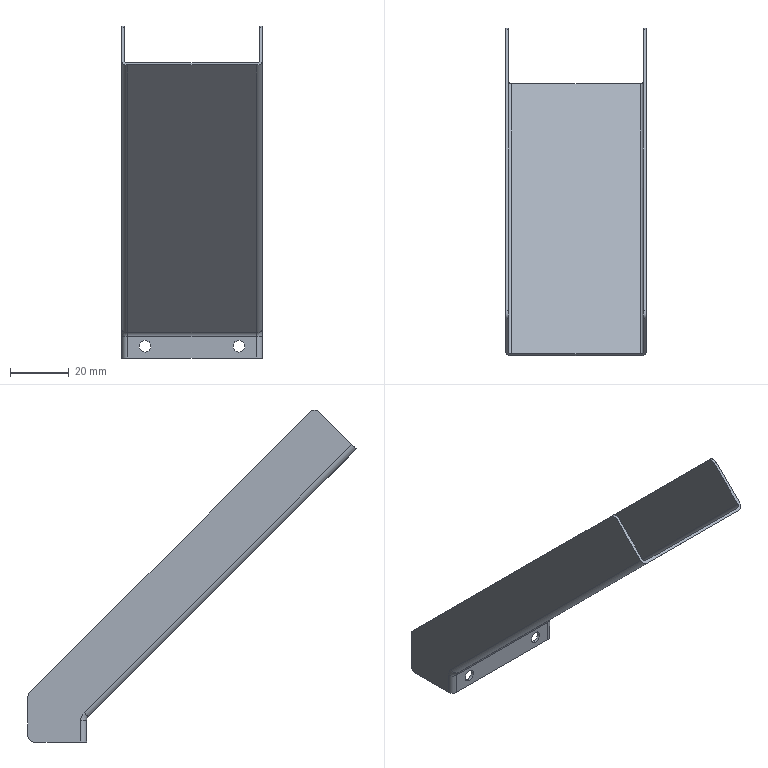Part | NX | features BREP 1 | 1 solid | 35 faces | box 48 x 112 x 113.314 mm | volume 12025 mm3 | cylinder 19 | plane 14 | torus 2 | commonest cylinder face diameters 4 x15 2 x4
STEP:
#1=CARTESIAN_POINT('',(40.,1.,6.));
#2=VERTEX_POINT('',#1);
#3=CARTESIAN_POINT('',(40.,1.,2.));
#4=VERTEX_POINT('',#3);
#5=CARTESIAN_POINT('',(40.,1.,4.));
#6=DIRECTION('',(0.,-1.,0.));
#7=DIRECTION('',(0.,0.,-1.));
#8=AXIS2_PLACEMENT_3D('',#5,#6,#7);
#9=CIRCLE('',#8,2.);
#10=EDGE_CURVE('',#2,#4,#9,.T.);
#11=ORIENTED_EDGE('',*,*,#10,.F.);
#12=CARTESIAN_POINT('',(40.,0.,6.));
#13=VERTEX_POINT('',#12);
#14=CARTESIAN_POINT('',(40.,0.,6.));
#15=DIRECTION('',(0.,-1.,0.));
#16=VECTOR('',#15,1000.);
#17=LINE('',#14,#16);
#18=EDGE_CURVE('',#2,#13,#17,.T.);
#19=ORIENTED_EDGE('',*,*,#18,.T.);
#20=CARTESIAN_POINT('',(40.,0.,2.));
#21=VERTEX_POINT('',#20);
#22=CARTESIAN_POINT('',(40.,0.,4.));
#23=DIRECTION('',(0.,-1.,0.));
#24=DIRECTION('',(0.,0.,-1.));
#25=AXIS2_PLACEMENT_3D('',#22,#23,#24);
#26=CIRCLE('',#25,2.);
#27=EDGE_CURVE('',#13,#21,#26,.T.);
#28=ORIENTED_EDGE('',*,*,#27,.T.);
#29=CARTESIAN_POINT('',(40.,0.,2.));
#30=DIRECTION('',(0.,-1.,0.));
#31=VECTOR('',#30,1000.);
#32=LINE('',#29,#31);
#33=EDGE_CURVE('',#4,#21,#32,.T.);
#34=ORIENTED_EDGE('',*,*,#33,.F.);
#35=EDGE_LOOP('',(#11,#19,#28,#34));
#36=FACE_BOUND('',#35,.T.);
#37=CARTESIAN_POINT('',(40.,0.,4.));
#38=DIRECTION('',(0.,-1.,0.));
#39=DIRECTION('',(0.,0.,-1.));
#40=AXIS2_PLACEMENT_3D('',#37,#38,#39);
#41=CYLINDRICAL_SURFACE('',#40,2.);
#42=ADVANCED_FACE('',(#36),#41,.F.);
#43=CARTESIAN_POINT('',(8.,1.,6.));
#44=VERTEX_POINT('',#43);
#45=CARTESIAN_POINT('',(8.,1.,2.));
#46=VERTEX_POINT('',#45);
#47=CARTESIAN_POINT('',(8.,1.,4.));
#48=DIRECTION('',(0.,-1.,0.));
#49=DIRECTION('',(0.,0.,-1.));
#50=AXIS2_PLACEMENT_3D('',#47,#48,#49);
#51=CIRCLE('',#50,2.);
#52=EDGE_CURVE('',#44,#46,#51,.T.);
#53=ORIENTED_EDGE('',*,*,#52,.F.);
#54=CARTESIAN_POINT('',(8.,0.,6.));
#55=VERTEX_POINT('',#54);
#56=CARTESIAN_POINT('',(8.,0.,6.));
#57=DIRECTION('',(0.,-1.,0.));
#58=VECTOR('',#57,1000.);
#59=LINE('',#56,#58);
#60=EDGE_CURVE('',#44,#55,#59,.T.);
#61=ORIENTED_EDGE('',*,*,#60,.T.);
#62=CARTESIAN_POINT('',(8.,0.,2.));
#63=VERTEX_POINT('',#62);
#64=CARTESIAN_POINT('',(8.,0.,4.));
#65=DIRECTION('',(0.,-1.,0.));
#66=DIRECTION('',(0.,0.,-1.));
#67=AXIS2_PLACEMENT_3D('',#64,#65,#66);
#68=CIRCLE('',#67,2.);
#69=EDGE_CURVE('',#55,#63,#68,.T.);
#70=ORIENTED_EDGE('',*,*,#69,.T.);
#71=CARTESIAN_POINT('',(8.,0.,2.));
#72=DIRECTION('',(0.,-1.,0.));
#73=VECTOR('',#72,1000.);
#74=LINE('',#71,#73);
#75=EDGE_CURVE('',#46,#63,#74,.T.);
#76=ORIENTED_EDGE('',*,*,#75,.F.);
#77=EDGE_LOOP('',(#53,#61,#70,#76));
#78=FACE_BOUND('',#77,.T.);
#79=CARTESIAN_POINT('',(8.,0.,4.));
#80=DIRECTION('',(0.,-1.,0.));
#81=DIRECTION('',(0.,0.,-1.));
#82=AXIS2_PLACEMENT_3D('',#79,#80,#81);
#83=CYLINDRICAL_SURFACE('',#82,2.);
#84=ADVANCED_FACE('',(#78),#83,.F.);
#85=CARTESIAN_POINT('',(46.,-92.,100.));
#86=VERTEX_POINT('',#85);
#87=CARTESIAN_POINT('',(2.,-92.,100.));
#88=VERTEX_POINT('',#87);
#89=CARTESIAN_POINT('',(0.,-92.,100.));
#90=DIRECTION('',(-1.,0.,0.));
#91=VECTOR('',#90,1000.);
#92=LINE('',#89,#91);
#93=EDGE_CURVE('',#86,#88,#92,.T.);
#94=ORIENTED_EDGE('',*,*,#93,.T.);
#95=CARTESIAN_POINT('',(2.,-0.5858,8.586));
#96=VERTEX_POINT('',#95);
#97=CARTESIAN_POINT('',(2.,0.,8.));
#98=DIRECTION('',(0.,0.7071,-0.7071));
#99=VECTOR('',#98,1000.);
#100=LINE('',#97,#99);
#101=EDGE_CURVE('',#88,#96,#100,.T.);
#102=ORIENTED_EDGE('',*,*,#101,.T.);
#103=CARTESIAN_POINT('',(46.,-0.5858,8.586));
#104=VERTEX_POINT('',#103);
#105=CARTESIAN_POINT('',(0.,-0.5858,8.586));
#106=DIRECTION('',(1.,0.,0.));
#107=VECTOR('',#106,1000.);
#108=LINE('',#105,#107);
#109=EDGE_CURVE('',#96,#104,#108,.T.);
#110=ORIENTED_EDGE('',*,*,#109,.T.);
#111=CARTESIAN_POINT('',(46.,-92.,100.));
#112=DIRECTION('',(0.,-0.7071,0.7071));
#113=VECTOR('',#112,1000.);
#114=LINE('',#111,#113);
#115=EDGE_CURVE('',#104,#86,#114,.T.);
#116=ORIENTED_EDGE('',*,*,#115,.T.);
#117=EDGE_LOOP('',(#94,#102,#110,#116));
#118=FACE_BOUND('',#117,.T.);
#119=CARTESIAN_POINT('',(0.,0.,8.));
#120=DIRECTION('',(0.,-0.7071,-0.7071));
#121=DIRECTION('',(0.,-0.7071,0.7071));
#122=AXIS2_PLACEMENT_3D('',#119,#120,#121);
#123=PLANE('',#122);
#124=ADVANCED_FACE('',(#118),#123,.T.);
#125=CARTESIAN_POINT('',(0.,19.414,16.87));
#126=VERTEX_POINT('',#125);
#127=CARTESIAN_POINT('',(0.,-76.444,112.728));
#128=VERTEX_POINT('',#127);
#129=CARTESIAN_POINT('',(0.,20.,16.284));
#130=DIRECTION('',(0.,-0.7071,0.7071));
#131=VECTOR('',#130,1000.);
#132=LINE('',#129,#131);
#133=EDGE_CURVE('',#126,#128,#132,.T.);
#134=ORIENTED_EDGE('',*,*,#133,.T.);
#135=CARTESIAN_POINT('',(1.,-76.444,112.728));
#136=VERTEX_POINT('',#135);
#137=CARTESIAN_POINT('',(0.,-76.444,112.728));
#138=DIRECTION('',(1.,0.,0.));
#139=VECTOR('',#138,1000.);
#140=LINE('',#137,#139);
#141=EDGE_CURVE('',#128,#136,#140,.T.);
#142=ORIENTED_EDGE('',*,*,#141,.T.);
#143=CARTESIAN_POINT('',(1.,19.414,16.87));
#144=VERTEX_POINT('',#143);
#145=CARTESIAN_POINT('',(1.,20.,16.284));
#146=DIRECTION('',(0.,-0.7071,0.7071));
#147=VECTOR('',#146,1000.);
#148=LINE('',#145,#147);
#149=EDGE_CURVE('',#144,#136,#148,.T.);
#150=ORIENTED_EDGE('',*,*,#149,.F.);
#151=CARTESIAN_POINT('',(0.,19.414,16.87));
#152=DIRECTION('',(-1.,0.,0.));
#153=VECTOR('',#152,1000.);
#154=LINE('',#151,#153);
#155=EDGE_CURVE('',#144,#126,#154,.T.);
#156=ORIENTED_EDGE('',*,*,#155,.T.);
#157=EDGE_LOOP('',(#134,#142,#150,#156));
#158=FACE_BOUND('',#157,.T.);
#159=CARTESIAN_POINT('',(0.,20.,16.284));
#160=DIRECTION('',(0.,0.7071,0.7071));
#161=DIRECTION('',(1.,0.,0.));
#162=AXIS2_PLACEMENT_3D('',#159,#160,#161);
#163=PLANE('',#162);
#164=ADVANCED_FACE('',(#158),#163,.T.);
#165=CARTESIAN_POINT('',(2.,-91.293,100.707));
#166=VERTEX_POINT('',#165);
#167=CARTESIAN_POINT('',(46.,-91.293,100.707));
#168=VERTEX_POINT('',#167);
#169=CARTESIAN_POINT('',(1.,-91.293,100.707));
#170=DIRECTION('',(1.,0.,0.));
#171=VECTOR('',#170,1000.);
#172=LINE('',#169,#171);
#173=EDGE_CURVE('',#166,#168,#172,.T.);
#174=ORIENTED_EDGE('',*,*,#173,.T.);
#175=CARTESIAN_POINT('',(46.,1.,8.414));
#176=VERTEX_POINT('',#175);
#177=CARTESIAN_POINT('',(46.,1.,8.414));
#178=DIRECTION('',(0.,0.7071,-0.7071));
#179=VECTOR('',#178,1000.);
#180=LINE('',#177,#179);
#181=EDGE_CURVE('',#168,#176,#180,.T.);
#182=ORIENTED_EDGE('',*,*,#181,.T.);
#183=CARTESIAN_POINT('',(2.,1.,8.414));
#184=VERTEX_POINT('',#183);
#185=CARTESIAN_POINT('',(1.,1.,8.414));
#186=DIRECTION('',(-1.,0.,0.));
#187=VECTOR('',#186,1000.);
#188=LINE('',#185,#187);
#189=EDGE_CURVE('',#176,#184,#188,.T.);
#190=ORIENTED_EDGE('',*,*,#189,.T.);
#191=CARTESIAN_POINT('',(2.,1.,8.414));
#192=DIRECTION('',(0.,-0.7071,0.7071));
#193=VECTOR('',#192,1000.);
#194=LINE('',#191,#193);
#195=EDGE_CURVE('',#184,#166,#194,.T.);
#196=ORIENTED_EDGE('',*,*,#195,.T.);
#197=EDGE_LOOP('',(#174,#182,#190,#196));
#198=FACE_BOUND('',#197,.T.);
#199=CARTESIAN_POINT('',(1.,1.,8.414));
#200=DIRECTION('',(0.,0.7071,0.7071));
#201=DIRECTION('',(1.,0.,0.));
#202=AXIS2_PLACEMENT_3D('',#199,#200,#201);
#203=PLANE('',#202);
#204=ADVANCED_FACE('',(#198),#203,.T.);
#205=CARTESIAN_POINT('',(47.,19.414,16.87));
#206=VERTEX_POINT('',#205);
#207=CARTESIAN_POINT('',(47.,-76.444,112.728));
#208=VERTEX_POINT('',#207);
#209=CARTESIAN_POINT('',(47.,20.,16.284));
#210=DIRECTION('',(0.,-0.7071,0.7071));
#211=VECTOR('',#210,1000.);
#212=LINE('',#209,#211);
#213=EDGE_CURVE('',#206,#208,#212,.T.);
#214=ORIENTED_EDGE('',*,*,#213,.T.);
#215=CARTESIAN_POINT('',(48.,-76.444,112.728));
#216=VERTEX_POINT('',#215);
#217=CARTESIAN_POINT('',(47.,-76.444,112.728));
#218=DIRECTION('',(1.,0.,0.));
#219=VECTOR('',#218,1000.);
#220=LINE('',#217,#219);
#221=EDGE_CURVE('',#208,#216,#220,.T.);
#222=ORIENTED_EDGE('',*,*,#221,.T.);
#223=CARTESIAN_POINT('',(48.,19.414,16.87));
#224=VERTEX_POINT('',#223);
#225=CARTESIAN_POINT('',(48.,20.,16.284));
#226=DIRECTION('',(0.,-0.7071,0.7071));
#227=VECTOR('',#226,1000.);
#228=LINE('',#225,#227);
#229=EDGE_CURVE('',#224,#216,#228,.T.);
#230=ORIENTED_EDGE('',*,*,#229,.F.);
#231=CARTESIAN_POINT('',(47.,19.414,16.87));
#232=DIRECTION('',(-1.,0.,0.));
#233=VECTOR('',#232,1000.);
#234=LINE('',#231,#233);
#235=EDGE_CURVE('',#224,#206,#234,.T.);
#236=ORIENTED_EDGE('',*,*,#235,.T.);
#237=EDGE_LOOP('',(#214,#222,#230,#236));
#238=FACE_BOUND('',#237,.T.);
#239=CARTESIAN_POINT('',(47.,20.,16.284));
#240=DIRECTION('',(0.,0.7071,0.7071));
#241=DIRECTION('',(1.,0.,0.));
#242=AXIS2_PLACEMENT_3D('',#239,#240,#241);
#243=PLANE('',#242);
#244=ADVANCED_FACE('',(#238),#243,.T.);
#245=CARTESIAN_POINT('',(46.,0.,7.172));
#246=VERTEX_POINT('',#245);
#247=CARTESIAN_POINT('',(2.,0.,7.172));
#248=VERTEX_POINT('',#247);
#249=CARTESIAN_POINT('',(0.,0.,7.172));
#250=DIRECTION('',(-1.,0.,0.));
#251=VECTOR('',#250,1000.);
#252=LINE('',#249,#251);
#253=EDGE_CURVE('',#246,#248,#252,.T.);
#254=ORIENTED_EDGE('',*,*,#253,.T.);
#255=CARTESIAN_POINT('',(2.,0.,0.));
#256=VERTEX_POINT('',#255);
#257=CARTESIAN_POINT('',(2.,0.,64.142));
#258=DIRECTION('',(0.,0.,-1.));
#259=VECTOR('',#258,1000.);
#260=LINE('',#257,#259);
#261=EDGE_CURVE('',#248,#256,#260,.T.);
#262=ORIENTED_EDGE('',*,*,#261,.T.);
#263=CARTESIAN_POINT('',(46.,0.,0.));
#264=VERTEX_POINT('',#263);
#265=CARTESIAN_POINT('',(0.,0.,0.));
#266=DIRECTION('',(1.,0.,0.));
#267=VECTOR('',#266,1000.);
#268=LINE('',#265,#267);
#269=EDGE_CURVE('',#256,#264,#268,.T.);
#270=ORIENTED_EDGE('',*,*,#269,.T.);
#271=CARTESIAN_POINT('',(46.,0.,64.142));
#272=DIRECTION('',(0.,0.,1.));
#273=VECTOR('',#272,1000.);
#274=LINE('',#271,#273);
#275=EDGE_CURVE('',#264,#246,#274,.T.);
#276=ORIENTED_EDGE('',*,*,#275,.T.);
#277=EDGE_LOOP('',(#254,#262,#270,#276));
#278=FACE_BOUND('',#277,.T.);
#279=CARTESIAN_POINT('',(40.,0.,4.));
#280=DIRECTION('',(0.,-1.,0.));
#281=DIRECTION('',(0.,0.,-1.));
#282=AXIS2_PLACEMENT_3D('',#279,#280,#281);
#283=CIRCLE('',#282,2.);
#284=EDGE_CURVE('',#21,#13,#283,.T.);
#285=ORIENTED_EDGE('',*,*,#284,.F.);
#286=ORIENTED_EDGE('',*,*,#27,.F.);
#287=EDGE_LOOP('',(#285,#286));
#288=FACE_BOUND('',#287,.T.);
#289=CARTESIAN_POINT('',(8.,0.,4.));
#290=DIRECTION('',(0.,-1.,0.));
#291=DIRECTION('',(0.,0.,-1.));
#292=AXIS2_PLACEMENT_3D('',#289,#290,#291);
#293=CIRCLE('',#292,2.);
#294=EDGE_CURVE('',#63,#55,#293,.T.);
#295=ORIENTED_EDGE('',*,*,#294,.F.);
#296=ORIENTED_EDGE('',*,*,#69,.F.);
#297=EDGE_LOOP('',(#295,#296));
#298=FACE_BOUND('',#297,.T.);
#299=CARTESIAN_POINT('',(0.,0.,64.142));
#300=DIRECTION('',(0.,1.,0.));
#301=DIRECTION('',(0.,0.,-1.));
#302=AXIS2_PLACEMENT_3D('',#299,#300,#301);
#303=PLANE('',#302);
#304=ADVANCED_FACE('',(#278,#288,#298),#303,.F.);
#305=CARTESIAN_POINT('',(48.,2.,7.172));
#306=VERTEX_POINT('',#305);
#307=CARTESIAN_POINT('',(48.,0.8284,10.));
#308=VERTEX_POINT('',#307);
#309=CARTESIAN_POINT('',(48.,-2.,7.172));
#310=DIRECTION('',(1.,0.,0.));
#311=DIRECTION('',(0.,0.,1.));
#312=AXIS2_PLACEMENT_3D('',#309,#310,#311);
#313=CIRCLE('',#312,4.);
#314=EDGE_CURVE('',#306,#308,#313,.T.);
#315=ORIENTED_EDGE('',*,*,#314,.F.);
#316=CARTESIAN_POINT('',(48.,2.,0.));
#317=VERTEX_POINT('',#316);
#318=CARTESIAN_POINT('',(48.,2.,64.142));
#319=DIRECTION('',(0.,0.,-1.));
#320=VECTOR('',#319,1000.);
#321=LINE('',#318,#320);
#322=EDGE_CURVE('',#306,#317,#321,.T.);
#323=ORIENTED_EDGE('',*,*,#322,.T.);
#324=CARTESIAN_POINT('',(48.,18.,0.));
#325=VERTEX_POINT('',#324);
#326=CARTESIAN_POINT('',(48.,0.,0.));
#327=DIRECTION('',(0.,1.,0.));
#328=VECTOR('',#327,1000.);
#329=LINE('',#326,#328);
#330=EDGE_CURVE('',#317,#325,#329,.T.);
#331=ORIENTED_EDGE('',*,*,#330,.T.);
#332=CARTESIAN_POINT('',(48.,20.,2.));
#333=VERTEX_POINT('',#332);
#334=CARTESIAN_POINT('',(48.,18.,2.));
#335=DIRECTION('',(1.,0.,0.));
#336=DIRECTION('',(0.,0.,1.));
#337=AXIS2_PLACEMENT_3D('',#334,#335,#336);
#338=CIRCLE('',#337,2.);
#339=EDGE_CURVE('',#325,#333,#338,.T.);
#340=ORIENTED_EDGE('',*,*,#339,.T.);
#341=CARTESIAN_POINT('',(48.,20.,15.456));
#342=VERTEX_POINT('',#341);
#343=CARTESIAN_POINT('',(48.,20.,64.142));
#344=DIRECTION('',(0.,0.,-1.));
#345=VECTOR('',#344,1000.);
#346=LINE('',#343,#345);
#347=EDGE_CURVE('',#342,#333,#346,.T.);
#348=ORIENTED_EDGE('',*,*,#347,.F.);
#349=CARTESIAN_POINT('',(48.,18.,15.456));
#350=DIRECTION('',(1.,0.,0.));
#351=DIRECTION('',(0.,0.,1.));
#352=AXIS2_PLACEMENT_3D('',#349,#350,#351);
#353=CIRCLE('',#352,2.);
#354=EDGE_CURVE('',#342,#224,#353,.T.);
#355=ORIENTED_EDGE('',*,*,#354,.T.);
#356=ORIENTED_EDGE('',*,*,#229,.T.);
#357=CARTESIAN_POINT('',(48.,-79.272,112.728));
#358=VERTEX_POINT('',#357);
#359=CARTESIAN_POINT('',(48.,-77.858,111.314));
#360=DIRECTION('',(1.,0.,0.));
#361=DIRECTION('',(0.,0.,1.));
#362=AXIS2_PLACEMENT_3D('',#359,#360,#361);
#363=CIRCLE('',#362,2.);
#364=EDGE_CURVE('',#216,#358,#363,.T.);
#365=ORIENTED_EDGE('',*,*,#364,.T.);
#366=CARTESIAN_POINT('',(48.,-90.586,101.414));
#367=VERTEX_POINT('',#366);
#368=CARTESIAN_POINT('',(48.,-77.964,114.036));
#369=DIRECTION('',(0.,-0.7071,-0.7071));
#370=VECTOR('',#369,1000.);
#371=LINE('',#368,#370);
#372=EDGE_CURVE('',#358,#367,#371,.T.);
#373=ORIENTED_EDGE('',*,*,#372,.T.);
#374=CARTESIAN_POINT('',(48.,1.414,9.414));
#375=DIRECTION('',(0.,0.7071,-0.7071));
#376=VECTOR('',#375,1000.);
#377=LINE('',#374,#376);
#378=EDGE_CURVE('',#367,#308,#377,.T.);
#379=ORIENTED_EDGE('',*,*,#378,.T.);
#380=EDGE_LOOP('',(#315,#323,#331,#340,#348,#355,#356,#365,#373,#379));
#381=FACE_BOUND('',#380,.T.);
#382=CARTESIAN_POINT('',(48.,0.,64.142));
#383=DIRECTION('',(-1.,0.,0.));
#384=DIRECTION('',(0.,0.,1.));
#385=AXIS2_PLACEMENT_3D('',#382,#383,#384);
#386=PLANE('',#385);
#387=ADVANCED_FACE('',(#381),#386,.F.);
#388=ORIENTED_EDGE('',*,*,#347,.T.);
#389=CARTESIAN_POINT('',(47.,20.,2.));
#390=VERTEX_POINT('',#389);
#391=CARTESIAN_POINT('',(47.,20.,2.));
#392=DIRECTION('',(-1.,0.,0.));
#393=VECTOR('',#392,1000.);
#394=LINE('',#391,#393);
#395=EDGE_CURVE('',#333,#390,#394,.T.);
#396=ORIENTED_EDGE('',*,*,#395,.T.);
#397=CARTESIAN_POINT('',(47.,20.,15.456));
#398=VERTEX_POINT('',#397);
#399=CARTESIAN_POINT('',(47.,20.,64.142));
#400=DIRECTION('',(0.,0.,-1.));
#401=VECTOR('',#400,1000.);
#402=LINE('',#399,#401);
#403=EDGE_CURVE('',#398,#390,#402,.T.);
#404=ORIENTED_EDGE('',*,*,#403,.F.);
#405=CARTESIAN_POINT('',(48.,20.,15.456));
#406=DIRECTION('',(1.,0.,0.));
#407=VECTOR('',#406,1000.);
#408=LINE('',#405,#407);
#409=EDGE_CURVE('',#398,#342,#408,.T.);
#410=ORIENTED_EDGE('',*,*,#409,.T.);
#411=EDGE_LOOP('',(#388,#396,#404,#410));
#412=FACE_BOUND('',#411,.T.);
#413=CARTESIAN_POINT('',(47.,20.,64.142));
#414=DIRECTION('',(0.,-1.,0.));
#415=DIRECTION('',(0.,0.,-1.));
#416=AXIS2_PLACEMENT_3D('',#413,#414,#415);
#417=PLANE('',#416);
#418=ADVANCED_FACE('',(#412),#417,.F.);
#419=CARTESIAN_POINT('',(47.,-90.586,101.414));
#420=VERTEX_POINT('',#419);
#421=CARTESIAN_POINT('',(47.,-79.272,112.728));
#422=VERTEX_POINT('',#421);
#423=CARTESIAN_POINT('',(47.,-77.361,114.639));
#424=DIRECTION('',(0.,0.7071,0.7071));
#425=VECTOR('',#424,1000.);
#426=LINE('',#423,#425);
#427=EDGE_CURVE('',#420,#422,#426,.T.);
#428=ORIENTED_EDGE('',*,*,#427,.T.);
#429=CARTESIAN_POINT('',(47.,-77.858,111.314));
#430=DIRECTION('',(-1.,0.,0.));
#431=DIRECTION('',(0.,0.,-1.));
#432=AXIS2_PLACEMENT_3D('',#429,#430,#431);
#433=CIRCLE('',#432,2.);
#434=EDGE_CURVE('',#422,#208,#433,.T.);
#435=ORIENTED_EDGE('',*,*,#434,.T.);
#436=ORIENTED_EDGE('',*,*,#213,.F.);
#437=CARTESIAN_POINT('',(47.,18.,15.456));
#438=DIRECTION('',(-1.,0.,0.));
#439=DIRECTION('',(0.,0.,-1.));
#440=AXIS2_PLACEMENT_3D('',#437,#438,#439);
#441=CIRCLE('',#440,2.);
#442=EDGE_CURVE('',#206,#398,#441,.T.);
#443=ORIENTED_EDGE('',*,*,#442,.T.);
#444=ORIENTED_EDGE('',*,*,#403,.T.);
#445=CARTESIAN_POINT('',(47.,18.,0.));
#446=VERTEX_POINT('',#445);
#447=CARTESIAN_POINT('',(47.,18.,2.));
#448=DIRECTION('',(-1.,0.,0.));
#449=DIRECTION('',(0.,0.,-1.));
#450=AXIS2_PLACEMENT_3D('',#447,#448,#449);
#451=CIRCLE('',#450,2.);
#452=EDGE_CURVE('',#390,#446,#451,.T.);
#453=ORIENTED_EDGE('',*,*,#452,.T.);
#454=CARTESIAN_POINT('',(47.,2.,0.));
#455=VERTEX_POINT('',#454);
#456=CARTESIAN_POINT('',(47.,1.,0.));
#457=DIRECTION('',(0.,-1.,0.));
#458=VECTOR('',#457,1000.);
#459=LINE('',#456,#458);
#460=EDGE_CURVE('',#446,#455,#459,.T.);
#461=ORIENTED_EDGE('',*,*,#460,.T.);
#462=CARTESIAN_POINT('',(47.,2.,8.828));
#463=VERTEX_POINT('',#462);
#464=CARTESIAN_POINT('',(47.,2.,8.414));
#465=DIRECTION('',(0.,0.,1.));
#466=VECTOR('',#465,1000.);
#467=LINE('',#464,#466);
#468=EDGE_CURVE('',#455,#463,#467,.T.);
#469=ORIENTED_EDGE('',*,*,#468,.T.);
#470=CARTESIAN_POINT('',(47.,-26.157,36.985));
#471=DIRECTION('',(0.,-0.7071,0.7071));
#472=VECTOR('',#471,1000.);
#473=LINE('',#470,#472);
#474=EDGE_CURVE('',#463,#420,#473,.T.);
#475=ORIENTED_EDGE('',*,*,#474,.T.);
#476=EDGE_LOOP('',(#428,#435,#436,#443,#444,#453,#461,#469,#475));
#477=FACE_BOUND('',#476,.T.);
#478=CARTESIAN_POINT('',(47.,1.,64.142));
#479=DIRECTION('',(1.,0.,0.));
#480=DIRECTION('',(0.,1.,0.));
#481=AXIS2_PLACEMENT_3D('',#478,#479,#480);
#482=PLANE('',#481);
#483=ADVANCED_FACE('',(#477),#482,.F.);
#484=CARTESIAN_POINT('',(46.,1.,0.));
#485=VERTEX_POINT('',#484);
#486=CARTESIAN_POINT('',(2.,1.,0.));
#487=VERTEX_POINT('',#486);
#488=CARTESIAN_POINT('',(1.,1.,0.));
#489=DIRECTION('',(-1.,0.,0.));
#490=VECTOR('',#489,1000.);
#491=LINE('',#488,#490);
#492=EDGE_CURVE('',#485,#487,#491,.T.);
#493=ORIENTED_EDGE('',*,*,#492,.T.);
#494=CARTESIAN_POINT('',(2.,1.,8.414));
#495=DIRECTION('',(0.,0.,1.));
#496=VECTOR('',#495,1000.);
#497=LINE('',#494,#496);
#498=EDGE_CURVE('',#487,#184,#497,.T.);
#499=ORIENTED_EDGE('',*,*,#498,.T.);
#500=ORIENTED_EDGE('',*,*,#189,.F.);
#501=CARTESIAN_POINT('',(46.,1.,0.));
#502=DIRECTION('',(0.,0.,-1.));
#503=VECTOR('',#502,1000.);
#504=LINE('',#501,#503);
#505=EDGE_CURVE('',#176,#485,#504,.T.);
#506=ORIENTED_EDGE('',*,*,#505,.T.);
#507=EDGE_LOOP('',(#493,#499,#500,#506));
#508=FACE_BOUND('',#507,.T.);
#509=CARTESIAN_POINT('',(40.,1.,4.));
#510=DIRECTION('',(0.,-1.,0.));
#511=DIRECTION('',(0.,0.,-1.));
#512=AXIS2_PLACEMENT_3D('',#509,#510,#511);
#513=CIRCLE('',#512,2.);
#514=EDGE_CURVE('',#4,#2,#513,.T.);
#515=ORIENTED_EDGE('',*,*,#514,.T.);
#516=ORIENTED_EDGE('',*,*,#10,.T.);
#517=EDGE_LOOP('',(#515,#516));
#518=FACE_BOUND('',#517,.T.);
#519=CARTESIAN_POINT('',(8.,1.,4.));
#520=DIRECTION('',(0.,-1.,0.));
#521=DIRECTION('',(0.,0.,-1.));
#522=AXIS2_PLACEMENT_3D('',#519,#520,#521);
#523=CIRCLE('',#522,2.);
#524=EDGE_CURVE('',#46,#44,#523,.T.);
#525=ORIENTED_EDGE('',*,*,#524,.T.);
#526=ORIENTED_EDGE('',*,*,#52,.T.);
#527=EDGE_LOOP('',(#525,#526));
#528=FACE_BOUND('',#527,.T.);
#529=CARTESIAN_POINT('',(1.,1.,64.142));
#530=DIRECTION('',(0.,-1.,0.));
#531=DIRECTION('',(0.,0.,-1.));
#532=AXIS2_PLACEMENT_3D('',#529,#530,#531);
#533=PLANE('',#532);
#534=ADVANCED_FACE('',(#508,#518,#528),#533,.F.);
#535=ORIENTED_EDGE('',*,*,#149,.T.);
#536=CARTESIAN_POINT('',(1.,-79.272,112.728));
#537=VERTEX_POINT('',#536);
#538=CARTESIAN_POINT('',(1.,-77.858,111.314));
#539=DIRECTION('',(1.,0.,0.));
#540=DIRECTION('',(0.,0.,1.));
#541=AXIS2_PLACEMENT_3D('',#538,#539,#540);
#542=CIRCLE('',#541,2.);
#543=EDGE_CURVE('',#136,#537,#542,.T.);
#544=ORIENTED_EDGE('',*,*,#543,.T.);
#545=CARTESIAN_POINT('',(1.,-90.586,101.414));
#546=VERTEX_POINT('',#545);
#547=CARTESIAN_POINT('',(1.,-77.361,114.639));
#548=DIRECTION('',(0.,-0.7071,-0.7071));
#549=VECTOR('',#548,1000.);
#550=LINE('',#547,#549);
#551=EDGE_CURVE('',#537,#546,#550,.T.);
#552=ORIENTED_EDGE('',*,*,#551,.T.);
#553=CARTESIAN_POINT('',(1.,2.,8.828));
#554=VERTEX_POINT('',#553);
#555=CARTESIAN_POINT('',(1.,-26.157,36.985));
#556=DIRECTION('',(0.,0.7071,-0.7071));
#557=VECTOR('',#556,1000.);
#558=LINE('',#555,#557);
#559=EDGE_CURVE('',#546,#554,#558,.T.);
#560=ORIENTED_EDGE('',*,*,#559,.T.);
#561=CARTESIAN_POINT('',(1.,2.,0.));
#562=VERTEX_POINT('',#561);
#563=CARTESIAN_POINT('',(1.,2.,0.));
#564=DIRECTION('',(0.,0.,-1.));
#565=VECTOR('',#564,1000.);
#566=LINE('',#563,#565);
#567=EDGE_CURVE('',#554,#562,#566,.T.);
#568=ORIENTED_EDGE('',*,*,#567,.T.);
#569=CARTESIAN_POINT('',(1.,18.,0.));
#570=VERTEX_POINT('',#569);
#571=CARTESIAN_POINT('',(1.,1.,0.));
#572=DIRECTION('',(0.,1.,0.));
#573=VECTOR('',#572,1000.);
#574=LINE('',#571,#573);
#575=EDGE_CURVE('',#562,#570,#574,.T.);
#576=ORIENTED_EDGE('',*,*,#575,.T.);
#577=CARTESIAN_POINT('',(1.,20.,2.));
#578=VERTEX_POINT('',#577);
#579=CARTESIAN_POINT('',(1.,18.,2.));
#580=DIRECTION('',(1.,0.,0.));
#581=DIRECTION('',(0.,0.,1.));
#582=AXIS2_PLACEMENT_3D('',#579,#580,#581);
#583=CIRCLE('',#582,2.);
#584=EDGE_CURVE('',#570,#578,#583,.T.);
#585=ORIENTED_EDGE('',*,*,#584,.T.);
#586=CARTESIAN_POINT('',(1.,20.,15.456));
#587=VERTEX_POINT('',#586);
#588=CARTESIAN_POINT('',(1.,20.,64.142));
#589=DIRECTION('',(0.,0.,-1.));
#590=VECTOR('',#589,1000.);
#591=LINE('',#588,#590);
#592=EDGE_CURVE('',#587,#578,#591,.T.);
#593=ORIENTED_EDGE('',*,*,#592,.F.);
#594=CARTESIAN_POINT('',(1.,18.,15.456));
#595=DIRECTION('',(1.,0.,0.));
#596=DIRECTION('',(0.,0.,1.));
#597=AXIS2_PLACEMENT_3D('',#594,#595,#596);
#598=CIRCLE('',#597,2.);
#599=EDGE_CURVE('',#587,#144,#598,.T.);
#600=ORIENTED_EDGE('',*,*,#599,.T.);
#601=EDGE_LOOP('',(#535,#544,#552,#560,#568,#576,#585,#593,#600));
#602=FACE_BOUND('',#601,.T.);
#603=CARTESIAN_POINT('',(1.,1.,64.142));
#604=DIRECTION('',(-1.,0.,0.));
#605=DIRECTION('',(0.,0.,1.));
#606=AXIS2_PLACEMENT_3D('',#603,#604,#605);
#607=PLANE('',#606);
#608=ADVANCED_FACE('',(#602),#607,.F.);
#609=CARTESIAN_POINT('',(0.,20.,15.456));
#610=VERTEX_POINT('',#609);
#611=CARTESIAN_POINT('',(0.,20.,2.));
#612=VERTEX_POINT('',#611);
#613=CARTESIAN_POINT('',(0.,20.,64.142));
#614=DIRECTION('',(0.,0.,-1.));
#615=VECTOR('',#614,1000.);
#616=LINE('',#613,#615);
#617=EDGE_CURVE('',#610,#612,#616,.T.);
#618=ORIENTED_EDGE('',*,*,#617,.F.);
#619=CARTESIAN_POINT('',(1.,20.,15.456));
#620=DIRECTION('',(1.,0.,0.));
#621=VECTOR('',#620,1000.);
#622=LINE('',#619,#621);
#623=EDGE_CURVE('',#610,#587,#622,.T.);
#624=ORIENTED_EDGE('',*,*,#623,.T.);
#625=ORIENTED_EDGE('',*,*,#592,.T.);
#626=CARTESIAN_POINT('',(0.,20.,2.));
#627=DIRECTION('',(-1.,0.,0.));
#628=VECTOR('',#627,1000.);
#629=LINE('',#626,#628);
#630=EDGE_CURVE('',#578,#612,#629,.T.);
#631=ORIENTED_EDGE('',*,*,#630,.T.);
#632=EDGE_LOOP('',(#618,#624,#625,#631));
#633=FACE_BOUND('',#632,.T.);
#634=CARTESIAN_POINT('',(0.,20.,64.142));
#635=DIRECTION('',(0.,-1.,0.));
#636=DIRECTION('',(0.,0.,-1.));
#637=AXIS2_PLACEMENT_3D('',#634,#635,#636);
#638=PLANE('',#637);
#639=ADVANCED_FACE('',(#633),#638,.F.);
#640=CARTESIAN_POINT('',(0.,18.,0.));
#641=VERTEX_POINT('',#640);
#642=CARTESIAN_POINT('',(0.,2.,0.));
#643=VERTEX_POINT('',#642);
#644=CARTESIAN_POINT('',(0.,0.,0.));
#645=DIRECTION('',(0.,-1.,0.));
#646=VECTOR('',#645,1000.);
#647=LINE('',#644,#646);
#648=EDGE_CURVE('',#641,#643,#647,.T.);
#649=ORIENTED_EDGE('',*,*,#648,.T.);
#650=CARTESIAN_POINT('',(0.,2.,7.172));
#651=VERTEX_POINT('',#650);
#652=CARTESIAN_POINT('',(0.,2.,64.142));
#653=DIRECTION('',(0.,0.,1.));
#654=VECTOR('',#653,1000.);
#655=LINE('',#652,#654);
#656=EDGE_CURVE('',#643,#651,#655,.T.);
#657=ORIENTED_EDGE('',*,*,#656,.T.);
#658=CARTESIAN_POINT('',(0.,0.8284,10.));
#659=VERTEX_POINT('',#658);
#660=CARTESIAN_POINT('',(0.,-2.,7.172));
#661=DIRECTION('',(-1.,0.,0.));
#662=DIRECTION('',(0.,0.,-1.));
#663=AXIS2_PLACEMENT_3D('',#660,#661,#662);
#664=CIRCLE('',#663,4.);
#665=EDGE_CURVE('',#659,#651,#664,.T.);
#666=ORIENTED_EDGE('',*,*,#665,.F.);
#667=CARTESIAN_POINT('',(0.,-90.586,101.414));
#668=VERTEX_POINT('',#667);
#669=CARTESIAN_POINT('',(0.,-90.586,101.414));
#670=DIRECTION('',(0.,-0.7071,0.7071));
#671=VECTOR('',#670,1000.);
#672=LINE('',#669,#671);
#673=EDGE_CURVE('',#659,#668,#672,.T.);
#674=ORIENTED_EDGE('',*,*,#673,.T.);
#675=CARTESIAN_POINT('',(0.,-79.272,112.728));
#676=VERTEX_POINT('',#675);
#677=CARTESIAN_POINT('',(0.,-77.964,114.036));
#678=DIRECTION('',(0.,0.7071,0.7071));
#679=VECTOR('',#678,1000.);
#680=LINE('',#677,#679);
#681=EDGE_CURVE('',#668,#676,#680,.T.);
#682=ORIENTED_EDGE('',*,*,#681,.T.);
#683=CARTESIAN_POINT('',(0.,-77.858,111.314));
#684=DIRECTION('',(-1.,0.,0.));
#685=DIRECTION('',(0.,0.,-1.));
#686=AXIS2_PLACEMENT_3D('',#683,#684,#685);
#687=CIRCLE('',#686,2.);
#688=EDGE_CURVE('',#676,#128,#687,.T.);
#689=ORIENTED_EDGE('',*,*,#688,.T.);
#690=ORIENTED_EDGE('',*,*,#133,.F.);
#691=CARTESIAN_POINT('',(0.,18.,15.456));
#692=DIRECTION('',(-1.,0.,0.));
#693=DIRECTION('',(0.,0.,-1.));
#694=AXIS2_PLACEMENT_3D('',#691,#692,#693);
#695=CIRCLE('',#694,2.);
#696=EDGE_CURVE('',#126,#610,#695,.T.);
#697=ORIENTED_EDGE('',*,*,#696,.T.);
#698=ORIENTED_EDGE('',*,*,#617,.T.);
#699=CARTESIAN_POINT('',(0.,18.,2.));
#700=DIRECTION('',(-1.,0.,0.));
#701=DIRECTION('',(0.,0.,-1.));
#702=AXIS2_PLACEMENT_3D('',#699,#700,#701);
#703=CIRCLE('',#702,2.);
#704=EDGE_CURVE('',#612,#641,#703,.T.);
#705=ORIENTED_EDGE('',*,*,#704,.T.);
#706=EDGE_LOOP('',(#649,#657,#666,#674,#682,#689,#690,#697,#698,#705));
#707=FACE_BOUND('',#706,.T.);
#708=CARTESIAN_POINT('',(0.,0.,64.142));
#709=DIRECTION('',(1.,0.,0.));
#710=DIRECTION('',(0.,1.,0.));
#711=AXIS2_PLACEMENT_3D('',#708,#709,#710);
#712=PLANE('',#711);
#713=ADVANCED_FACE('',(#707),#712,.F.);
#714=ORIENTED_EDGE('',*,*,#269,.F.);
#715=CARTESIAN_POINT('',(2.,2.,0.));
#716=DIRECTION('',(0.,0.,-1.));
#717=DIRECTION('',(-1.,0.,0.));
#718=AXIS2_PLACEMENT_3D('',#715,#716,#717);
#719=CIRCLE('',#718,2.);
#720=EDGE_CURVE('',#256,#643,#719,.T.);
#721=ORIENTED_EDGE('',*,*,#720,.T.);
#722=ORIENTED_EDGE('',*,*,#648,.F.);
#723=CARTESIAN_POINT('',(1.,18.,0.));
#724=DIRECTION('',(1.,0.,0.));
#725=VECTOR('',#724,1000.);
#726=LINE('',#723,#725);
#727=EDGE_CURVE('',#641,#570,#726,.T.);
#728=ORIENTED_EDGE('',*,*,#727,.T.);
#729=ORIENTED_EDGE('',*,*,#575,.F.);
#730=CARTESIAN_POINT('',(2.,2.,0.));
#731=DIRECTION('',(0.,0.,1.));
#732=DIRECTION('',(-1.,0.,0.));
#733=AXIS2_PLACEMENT_3D('',#730,#731,#732);
#734=CIRCLE('',#733,1.);
#735=EDGE_CURVE('',#562,#487,#734,.T.);
#736=ORIENTED_EDGE('',*,*,#735,.T.);
#737=ORIENTED_EDGE('',*,*,#492,.F.);
#738=CARTESIAN_POINT('',(46.,2.,0.));
#739=DIRECTION('',(0.,0.,1.));
#740=DIRECTION('',(-1.,0.,0.));
#741=AXIS2_PLACEMENT_3D('',#738,#739,#740);
#742=CIRCLE('',#741,1.);
#743=EDGE_CURVE('',#485,#455,#742,.T.);
#744=ORIENTED_EDGE('',*,*,#743,.T.);
#745=ORIENTED_EDGE('',*,*,#460,.F.);
#746=CARTESIAN_POINT('',(48.,18.,0.));
#747=DIRECTION('',(1.,0.,0.));
#748=VECTOR('',#747,1000.);
#749=LINE('',#746,#748);
#750=EDGE_CURVE('',#446,#325,#749,.T.);
#751=ORIENTED_EDGE('',*,*,#750,.T.);
#752=ORIENTED_EDGE('',*,*,#330,.F.);
#753=CARTESIAN_POINT('',(46.,2.,0.));
#754=DIRECTION('',(0.,0.,-1.));
#755=DIRECTION('',(-1.,0.,0.));
#756=AXIS2_PLACEMENT_3D('',#753,#754,#755);
#757=CIRCLE('',#756,2.);
#758=EDGE_CURVE('',#317,#264,#757,.T.);
#759=ORIENTED_EDGE('',*,*,#758,.T.);
#760=EDGE_LOOP('',(#714,#721,#722,#728,#729,#736,#737,#744,#745,#751,#752,#759));
#761=FACE_BOUND('',#760,.T.);
#762=CARTESIAN_POINT('',(0.,0.,0.));
#763=DIRECTION('',(0.,0.,-1.));
#764=DIRECTION('',(0.,-1.,0.));
#765=AXIS2_PLACEMENT_3D('',#762,#763,#764);
#766=PLANE('',#765);
#767=ADVANCED_FACE('',(#761),#766,.T.);
#768=ORIENTED_EDGE('',*,*,#681,.F.);
#769=CARTESIAN_POINT('',(2.,-90.586,101.414));
#770=DIRECTION('',(0.,-0.7071,0.7071));
#771=DIRECTION('',(0.,-0.7071,-0.7071));
#772=AXIS2_PLACEMENT_3D('',#769,#770,#771);
#773=CIRCLE('',#772,2.);
#774=EDGE_CURVE('',#668,#88,#773,.T.);
#775=ORIENTED_EDGE('',*,*,#774,.T.);
#776=ORIENTED_EDGE('',*,*,#93,.F.);
#777=CARTESIAN_POINT('',(46.,-90.586,101.414));
#778=DIRECTION('',(0.,-0.7071,0.7071));
#779=DIRECTION('',(0.,-0.7071,-0.7071));
#780=AXIS2_PLACEMENT_3D('',#777,#778,#779);
#781=CIRCLE('',#780,2.);
#782=EDGE_CURVE('',#86,#367,#781,.T.);
#783=ORIENTED_EDGE('',*,*,#782,.T.);
#784=ORIENTED_EDGE('',*,*,#372,.F.);
#785=CARTESIAN_POINT('',(24.,-79.272,112.728));
#786=DIRECTION('',(-1.,0.,0.));
#787=VECTOR('',#786,1000.);
#788=LINE('',#785,#787);
#789=EDGE_CURVE('',#358,#422,#788,.T.);
#790=ORIENTED_EDGE('',*,*,#789,.T.);
#791=ORIENTED_EDGE('',*,*,#427,.F.);
#792=CARTESIAN_POINT('',(46.,-90.586,101.414));
#793=DIRECTION('',(0.,0.7071,-0.7071));
#794=DIRECTION('',(0.,-0.7071,-0.7071));
#795=AXIS2_PLACEMENT_3D('',#792,#793,#794);
#796=CIRCLE('',#795,1.);
#797=EDGE_CURVE('',#420,#168,#796,.T.);
#798=ORIENTED_EDGE('',*,*,#797,.T.);
#799=ORIENTED_EDGE('',*,*,#173,.F.);
#800=CARTESIAN_POINT('',(2.,-90.586,101.414));
#801=DIRECTION('',(0.,0.7071,-0.7071));
#802=DIRECTION('',(0.,-0.7071,-0.7071));
#803=AXIS2_PLACEMENT_3D('',#800,#801,#802);
#804=CIRCLE('',#803,1.);
#805=EDGE_CURVE('',#166,#546,#804,.T.);
#806=ORIENTED_EDGE('',*,*,#805,.T.);
#807=ORIENTED_EDGE('',*,*,#551,.F.);
#808=CARTESIAN_POINT('',(24.,-79.272,112.728));
#809=DIRECTION('',(-1.,0.,0.));
#810=VECTOR('',#809,1000.);
#811=LINE('',#808,#810);
#812=EDGE_CURVE('',#537,#676,#811,.T.);
#813=ORIENTED_EDGE('',*,*,#812,.T.);
#814=EDGE_LOOP('',(#768,#775,#776,#783,#784,#790,#791,#798,#799,#806,#807,#813));
#815=FACE_BOUND('',#814,.T.);
#816=CARTESIAN_POINT('',(24.,-84.929,107.071));
#817=DIRECTION('',(0.,-0.7071,0.7071));
#818=DIRECTION('',(-1.,0.,0.));
#819=AXIS2_PLACEMENT_3D('',#816,#817,#818);
#820=PLANE('',#819);
#821=ADVANCED_FACE('',(#815),#820,.T.);
#822=ORIENTED_EDGE('',*,*,#60,.F.);
#823=ORIENTED_EDGE('',*,*,#524,.F.);
#824=ORIENTED_EDGE('',*,*,#75,.T.);
#825=ORIENTED_EDGE('',*,*,#294,.T.);
#826=EDGE_LOOP('',(#822,#823,#824,#825));
#827=FACE_BOUND('',#826,.T.);
#828=CARTESIAN_POINT('',(8.,0.,4.));
#829=DIRECTION('',(0.,-1.,0.));
#830=DIRECTION('',(0.,0.,-1.));
#831=AXIS2_PLACEMENT_3D('',#828,#829,#830);
#832=CYLINDRICAL_SURFACE('',#831,2.);
#833=ADVANCED_FACE('',(#827),#832,.F.);
#834=ORIENTED_EDGE('',*,*,#18,.F.);
#835=ORIENTED_EDGE('',*,*,#514,.F.);
#836=ORIENTED_EDGE('',*,*,#33,.T.);
#837=ORIENTED_EDGE('',*,*,#284,.T.);
#838=EDGE_LOOP('',(#834,#835,#836,#837));
#839=FACE_BOUND('',#838,.T.);
#840=CARTESIAN_POINT('',(40.,0.,4.));
#841=DIRECTION('',(0.,-1.,0.));
#842=DIRECTION('',(0.,0.,-1.));
#843=AXIS2_PLACEMENT_3D('',#840,#841,#842);
#844=CYLINDRICAL_SURFACE('',#843,2.);
#845=ADVANCED_FACE('',(#839),#844,.F.);
#846=ORIENTED_EDGE('',*,*,#805,.F.);
#847=ORIENTED_EDGE('',*,*,#195,.F.);
#848=CARTESIAN_POINT('',(1.,2.,8.828));
#849=CARTESIAN_POINT('',(1.,1.414,8.586));
#850=CARTESIAN_POINT('',(1.414,1.,8.414));
#851=CARTESIAN_POINT('',(2.,1.,8.414));
#852=(BOUNDED_CURVE()B_SPLINE_CURVE(3,(#848,#849,#850,#851),.UNSPECIFIED.,.F.,.F.)B_SPLINE_CURVE_WITH_KNOTS((4,4),(4.712,6.283),.UNSPECIFIED.)CURVE()GEOMETRIC_REPRESENTATION_ITEM()RATIONAL_B_SPLINE_CURVE((1.,0.8047,0.8047,1.))REPRESENTATION_ITEM(''));
#853=EDGE_CURVE('',#554,#184,#852,.T.);
#854=ORIENTED_EDGE('',*,*,#853,.F.);
#855=ORIENTED_EDGE('',*,*,#559,.F.);
#856=EDGE_LOOP('',(#846,#847,#854,#855));
#857=FACE_BOUND('',#856,.T.);
#858=CARTESIAN_POINT('',(2.,1.707,9.121));
#859=DIRECTION('',(0.,-0.7071,0.7071));
#860=DIRECTION('',(0.,-0.7071,-0.7071));
#861=AXIS2_PLACEMENT_3D('',#858,#859,#860);
#862=CYLINDRICAL_SURFACE('',#861,1.);
#863=ADVANCED_FACE('',(#857),#862,.F.);
#864=ORIENTED_EDGE('',*,*,#853,.T.);
#865=ORIENTED_EDGE('',*,*,#498,.F.);
#866=ORIENTED_EDGE('',*,*,#735,.F.);
#867=ORIENTED_EDGE('',*,*,#567,.F.);
#868=EDGE_LOOP('',(#864,#865,#866,#867));
#869=FACE_BOUND('',#868,.T.);
#870=CARTESIAN_POINT('',(2.,2.,64.142));
#871=DIRECTION('',(0.,0.,1.));
#872=DIRECTION('',(0.,-1.,0.));
#873=AXIS2_PLACEMENT_3D('',#870,#871,#872);
#874=CYLINDRICAL_SURFACE('',#873,1.);
#875=ADVANCED_FACE('',(#869),#874,.F.);
#876=ORIENTED_EDGE('',*,*,#797,.F.);
#877=ORIENTED_EDGE('',*,*,#474,.F.);
#878=CARTESIAN_POINT('',(46.,1.,8.414));
#879=CARTESIAN_POINT('',(46.586,1.,8.414));
#880=CARTESIAN_POINT('',(47.,1.414,8.586));
#881=CARTESIAN_POINT('',(47.,2.,8.828));
#882=(BOUNDED_CURVE()B_SPLINE_CURVE(3,(#878,#879,#880,#881),.UNSPECIFIED.,.F.,.F.)B_SPLINE_CURVE_WITH_KNOTS((4,4),(0.,1.571),.UNSPECIFIED.)CURVE()GEOMETRIC_REPRESENTATION_ITEM()RATIONAL_B_SPLINE_CURVE((1.,0.8047,0.8047,1.))REPRESENTATION_ITEM(''));
#883=EDGE_CURVE('',#176,#463,#882,.T.);
#884=ORIENTED_EDGE('',*,*,#883,.F.);
#885=ORIENTED_EDGE('',*,*,#181,.F.);
#886=EDGE_LOOP('',(#876,#877,#884,#885));
#887=FACE_BOUND('',#886,.T.);
#888=CARTESIAN_POINT('',(46.,-26.157,36.985));
#889=DIRECTION('',(0.,-0.7071,0.7071));
#890=DIRECTION('',(0.,-0.7071,-0.7071));
#891=AXIS2_PLACEMENT_3D('',#888,#889,#890);
#892=CYLINDRICAL_SURFACE('',#891,1.);
#893=ADVANCED_FACE('',(#887),#892,.F.);
#894=ORIENTED_EDGE('',*,*,#883,.T.);
#895=ORIENTED_EDGE('',*,*,#468,.F.);
#896=ORIENTED_EDGE('',*,*,#743,.F.);
#897=ORIENTED_EDGE('',*,*,#505,.F.);
#898=EDGE_LOOP('',(#894,#895,#896,#897));
#899=FACE_BOUND('',#898,.T.);
#900=CARTESIAN_POINT('',(46.,2.,64.142));
#901=DIRECTION('',(0.,0.,1.));
#902=DIRECTION('',(0.,-1.,0.));
#903=AXIS2_PLACEMENT_3D('',#900,#901,#902);
#904=CYLINDRICAL_SURFACE('',#903,1.);
#905=ADVANCED_FACE('',(#899),#904,.F.);
#906=ORIENTED_EDGE('',*,*,#782,.F.);
#907=ORIENTED_EDGE('',*,*,#115,.F.);
#908=CARTESIAN_POINT('',(46.,0.8284,10.));
#909=DIRECTION('',(0.,0.7071,-0.7071));
#910=DIRECTION('',(0.,0.7071,0.7071));
#911=AXIS2_PLACEMENT_3D('',#908,#909,#910);
#912=CIRCLE('',#911,2.);
#913=EDGE_CURVE('',#308,#104,#912,.T.);
#914=ORIENTED_EDGE('',*,*,#913,.F.);
#915=ORIENTED_EDGE('',*,*,#378,.F.);
#916=EDGE_LOOP('',(#906,#907,#914,#915));
#917=FACE_BOUND('',#916,.T.);
#918=CARTESIAN_POINT('',(46.,1.414,9.414));
#919=DIRECTION('',(0.,0.7071,-0.7071));
#920=DIRECTION('',(0.,0.7071,0.7071));
#921=AXIS2_PLACEMENT_3D('',#918,#919,#920);
#922=CYLINDRICAL_SURFACE('',#921,2.);
#923=ADVANCED_FACE('',(#917),#922,.T.);
#924=ORIENTED_EDGE('',*,*,#758,.F.);
#925=ORIENTED_EDGE('',*,*,#322,.F.);
#926=CARTESIAN_POINT('',(46.,2.,7.172));
#927=DIRECTION('',(0.,0.,1.));
#928=DIRECTION('',(1.,0.,0.));
#929=AXIS2_PLACEMENT_3D('',#926,#927,#928);
#930=CIRCLE('',#929,2.);
#931=EDGE_CURVE('',#246,#306,#930,.T.);
#932=ORIENTED_EDGE('',*,*,#931,.F.);
#933=ORIENTED_EDGE('',*,*,#275,.F.);
#934=EDGE_LOOP('',(#924,#925,#932,#933));
#935=FACE_BOUND('',#934,.T.);
#936=CARTESIAN_POINT('',(46.,2.,64.142));
#937=DIRECTION('',(0.,0.,-1.));
#938=DIRECTION('',(0.,1.,0.));
#939=AXIS2_PLACEMENT_3D('',#936,#937,#938);
#940=CYLINDRICAL_SURFACE('',#939,2.);
#941=ADVANCED_FACE('',(#935),#940,.T.);
#942=ORIENTED_EDGE('',*,*,#314,.T.);
#943=ORIENTED_EDGE('',*,*,#913,.T.);
#944=CARTESIAN_POINT('',(46.,-2.,7.172));
#945=DIRECTION('',(1.,0.,0.));
#946=DIRECTION('',(0.,0.,1.));
#947=AXIS2_PLACEMENT_3D('',#944,#945,#946);
#948=CIRCLE('',#947,2.);
#949=EDGE_CURVE('',#246,#104,#948,.T.);
#950=ORIENTED_EDGE('',*,*,#949,.F.);
#951=ORIENTED_EDGE('',*,*,#931,.T.);
#952=EDGE_LOOP('',(#942,#943,#950,#951));
#953=FACE_BOUND('',#952,.T.);
#954=CARTESIAN_POINT('',(46.,-2.,7.172));
#955=DIRECTION('',(-1.,0.,0.));
#956=DIRECTION('',(0.,0.,1.));
#957=AXIS2_PLACEMENT_3D('',#954,#955,#956);
#958=TOROIDAL_SURFACE('',#957,4.,2.);
#959=ADVANCED_FACE('',(#953),#958,.T.);
#960=ORIENTED_EDGE('',*,*,#774,.F.);
#961=ORIENTED_EDGE('',*,*,#673,.F.);
#962=CARTESIAN_POINT('',(2.,0.8284,10.));
#963=DIRECTION('',(0.,0.7071,-0.7071));
#964=DIRECTION('',(0.,0.7071,0.7071));
#965=AXIS2_PLACEMENT_3D('',#962,#963,#964);
#966=CIRCLE('',#965,2.);
#967=EDGE_CURVE('',#96,#659,#966,.T.);
#968=ORIENTED_EDGE('',*,*,#967,.F.);
#969=ORIENTED_EDGE('',*,*,#101,.F.);
#970=EDGE_LOOP('',(#960,#961,#968,#969));
#971=FACE_BOUND('',#970,.T.);
#972=CARTESIAN_POINT('',(2.,-26.657,37.485));
#973=DIRECTION('',(0.,0.7071,-0.7071));
#974=DIRECTION('',(0.,0.7071,0.7071));
#975=AXIS2_PLACEMENT_3D('',#972,#973,#974);
#976=CYLINDRICAL_SURFACE('',#975,2.);
#977=ADVANCED_FACE('',(#971),#976,.T.);
#978=ORIENTED_EDGE('',*,*,#949,.T.);
#979=ORIENTED_EDGE('',*,*,#109,.F.);
#980=CARTESIAN_POINT('',(2.,-2.,7.172));
#981=DIRECTION('',(1.,0.,0.));
#982=DIRECTION('',(0.,0.,-1.));
#983=AXIS2_PLACEMENT_3D('',#980,#981,#982);
#984=CIRCLE('',#983,2.);
#985=EDGE_CURVE('',#248,#96,#984,.T.);
#986=ORIENTED_EDGE('',*,*,#985,.F.);
#987=ORIENTED_EDGE('',*,*,#253,.F.);
#988=EDGE_LOOP('',(#978,#979,#986,#987));
#989=FACE_BOUND('',#988,.T.);
#990=CARTESIAN_POINT('',(0.,-2.,7.172));
#991=DIRECTION('',(1.,0.,0.));
#992=DIRECTION('',(0.,0.,-1.));
#993=AXIS2_PLACEMENT_3D('',#990,#991,#992);
#994=CYLINDRICAL_SURFACE('',#993,2.);
#995=ADVANCED_FACE('',(#989),#994,.F.);
#996=ORIENTED_EDGE('',*,*,#967,.T.);
#997=ORIENTED_EDGE('',*,*,#665,.T.);
#998=CARTESIAN_POINT('',(2.,2.,7.172));
#999=DIRECTION('',(0.,0.,-1.));
#1000=DIRECTION('',(1.,0.,0.));
#1001=AXIS2_PLACEMENT_3D('',#998,#999,#1000);
#1002=CIRCLE('',#1001,2.);
#1003=EDGE_CURVE('',#248,#651,#1002,.T.);
#1004=ORIENTED_EDGE('',*,*,#1003,.F.);
#1005=ORIENTED_EDGE('',*,*,#985,.T.);
#1006=EDGE_LOOP('',(#996,#997,#1004,#1005));
#1007=FACE_BOUND('',#1006,.T.);
#1008=CARTESIAN_POINT('',(2.,-2.,7.172));
#1009=DIRECTION('',(1.,0.,0.));
#1010=DIRECTION('',(0.,0.,-1.));
#1011=AXIS2_PLACEMENT_3D('',#1008,#1009,#1010);
#1012=TOROIDAL_SURFACE('',#1011,4.,2.);
#1013=ADVANCED_FACE('',(#1007),#1012,.T.);
#1014=ORIENTED_EDGE('',*,*,#1003,.T.);
#1015=ORIENTED_EDGE('',*,*,#656,.F.);
#1016=ORIENTED_EDGE('',*,*,#720,.F.);
#1017=ORIENTED_EDGE('',*,*,#261,.F.);
#1018=EDGE_LOOP('',(#1014,#1015,#1016,#1017));
#1019=FACE_BOUND('',#1018,.T.);
#1020=CARTESIAN_POINT('',(2.,2.,64.142));
#1021=DIRECTION('',(0.,0.,-1.));
#1022=DIRECTION('',(0.,1.,0.));
#1023=AXIS2_PLACEMENT_3D('',#1020,#1021,#1022);
#1024=CYLINDRICAL_SURFACE('',#1023,2.);
#1025=ADVANCED_FACE('',(#1019),#1024,.T.);
#1026=ORIENTED_EDGE('',*,*,#688,.F.);
#1027=ORIENTED_EDGE('',*,*,#812,.F.);
#1028=ORIENTED_EDGE('',*,*,#543,.F.);
#1029=ORIENTED_EDGE('',*,*,#141,.F.);
#1030=EDGE_LOOP('',(#1026,#1027,#1028,#1029));
#1031=FACE_BOUND('',#1030,.T.);
#1032=CARTESIAN_POINT('',(0.,-77.858,111.314));
#1033=DIRECTION('',(1.,0.,0.));
#1034=DIRECTION('',(0.,0.,-1.));
#1035=AXIS2_PLACEMENT_3D('',#1032,#1033,#1034);
#1036=CYLINDRICAL_SURFACE('',#1035,2.);
#1037=ADVANCED_FACE('',(#1031),#1036,.T.);
#1038=ORIENTED_EDGE('',*,*,#434,.F.);
#1039=ORIENTED_EDGE('',*,*,#789,.F.);
#1040=ORIENTED_EDGE('',*,*,#364,.F.);
#1041=ORIENTED_EDGE('',*,*,#221,.F.);
#1042=EDGE_LOOP('',(#1038,#1039,#1040,#1041));
#1043=FACE_BOUND('',#1042,.T.);
#1044=CARTESIAN_POINT('',(47.,-77.858,111.314));
#1045=DIRECTION('',(1.,0.,0.));
#1046=DIRECTION('',(0.,0.,-1.));
#1047=AXIS2_PLACEMENT_3D('',#1044,#1045,#1046);
#1048=CYLINDRICAL_SURFACE('',#1047,2.);
#1049=ADVANCED_FACE('',(#1043),#1048,.T.);
#1050=ORIENTED_EDGE('',*,*,#339,.F.);
#1051=ORIENTED_EDGE('',*,*,#750,.F.);
#1052=ORIENTED_EDGE('',*,*,#452,.F.);
#1053=ORIENTED_EDGE('',*,*,#395,.F.);
#1054=EDGE_LOOP('',(#1050,#1051,#1052,#1053));
#1055=FACE_BOUND('',#1054,.T.);
#1056=CARTESIAN_POINT('',(47.,18.,2.));
#1057=DIRECTION('',(1.,0.,0.));
#1058=DIRECTION('',(0.,0.,-1.));
#1059=AXIS2_PLACEMENT_3D('',#1056,#1057,#1058);
#1060=CYLINDRICAL_SURFACE('',#1059,2.);
#1061=ADVANCED_FACE('',(#1055),#1060,.T.);
#1062=ORIENTED_EDGE('',*,*,#354,.F.);
#1063=ORIENTED_EDGE('',*,*,#409,.F.);
#1064=ORIENTED_EDGE('',*,*,#442,.F.);
#1065=ORIENTED_EDGE('',*,*,#235,.F.);
#1066=EDGE_LOOP('',(#1062,#1063,#1064,#1065));
#1067=FACE_BOUND('',#1066,.T.);
#1068=CARTESIAN_POINT('',(47.,18.,15.456));
#1069=DIRECTION('',(1.,0.,0.));
#1070=DIRECTION('',(0.,0.,-1.));
#1071=AXIS2_PLACEMENT_3D('',#1068,#1069,#1070);
#1072=CYLINDRICAL_SURFACE('',#1071,2.);
#1073=ADVANCED_FACE('',(#1067),#1072,.T.);
#1074=ORIENTED_EDGE('',*,*,#599,.F.);
#1075=ORIENTED_EDGE('',*,*,#623,.F.);
#1076=ORIENTED_EDGE('',*,*,#696,.F.);
#1077=ORIENTED_EDGE('',*,*,#155,.F.);
#1078=EDGE_LOOP('',(#1074,#1075,#1076,#1077));
#1079=FACE_BOUND('',#1078,.T.);
#1080=CARTESIAN_POINT('',(0.,18.,15.456));
#1081=DIRECTION('',(1.,0.,0.));
#1082=DIRECTION('',(0.,0.,-1.));
#1083=AXIS2_PLACEMENT_3D('',#1080,#1081,#1082);
#1084=CYLINDRICAL_SURFACE('',#1083,2.);
#1085=ADVANCED_FACE('',(#1079),#1084,.T.);
#1086=ORIENTED_EDGE('',*,*,#584,.F.);
#1087=ORIENTED_EDGE('',*,*,#727,.F.);
#1088=ORIENTED_EDGE('',*,*,#704,.F.);
#1089=ORIENTED_EDGE('',*,*,#630,.F.);
#1090=EDGE_LOOP('',(#1086,#1087,#1088,#1089));
#1091=FACE_BOUND('',#1090,.T.);
#1092=CARTESIAN_POINT('',(0.,18.,2.));
#1093=DIRECTION('',(1.,0.,0.));
#1094=DIRECTION('',(0.,0.,-1.));
#1095=AXIS2_PLACEMENT_3D('',#1092,#1093,#1094);
#1096=CYLINDRICAL_SURFACE('',#1095,2.);
#1097=ADVANCED_FACE('',(#1091),#1096,.T.);
#1098=CLOSED_SHELL('',(#42,#84,#124,#164,#204,#244,#304,#387,#418,#483,#534,#608,#639,#713,#767,#821,#833,#845,#863,#875,#893,#905,#923,#941,#959,#977,#995,#1013,#1025,#1037,#1049,#1061,#1073,#1085,#1097));
#1099=MANIFOLD_SOLID_BREP('',#1098);
#1100=(LENGTH_UNIT()NAMED_UNIT(*)SI_UNIT(.MILLI.,.METRE.));
#1101=UNCERTAINTY_MEASURE_WITH_UNIT(LENGTH_MEASURE(0.00001),#1100,'','');
#1102=(NAMED_UNIT(*)PLANE_ANGLE_UNIT()SI_UNIT($,.RADIAN.));
#1103=(NAMED_UNIT(*)SI_UNIT($,.STERADIAN.)SOLID_ANGLE_UNIT());
#1104=(GEOMETRIC_REPRESENTATION_CONTEXT(3)GLOBAL_UNCERTAINTY_ASSIGNED_CONTEXT((#1101))GLOBAL_UNIT_ASSIGNED_CONTEXT((#1100,#1102,#1103))REPRESENTATION_CONTEXT('',''));
#1105=ADVANCED_BREP_SHAPE_REPRESENTATION('',(#1099),#1104);